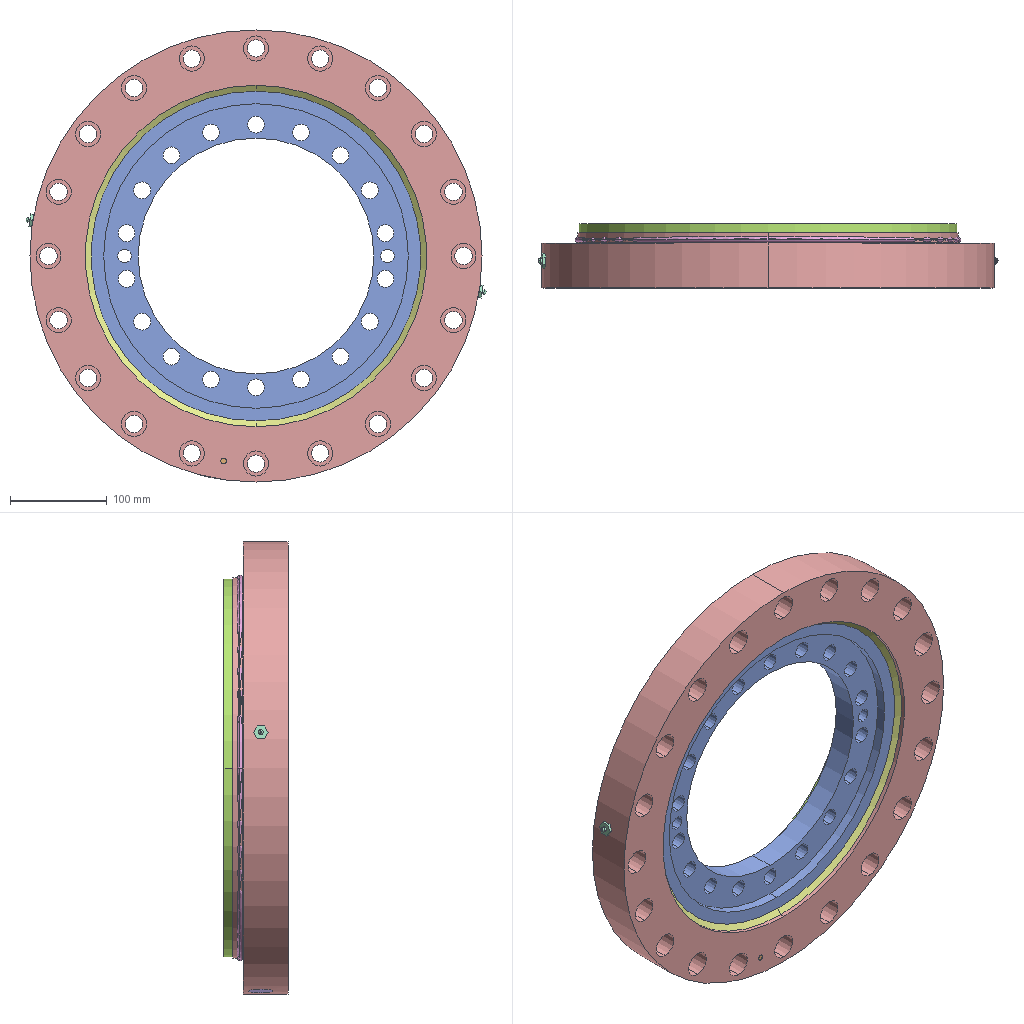Assembly | SolidWorks | 12 different items | 36 placed | box 474 x 66 x 466 mm
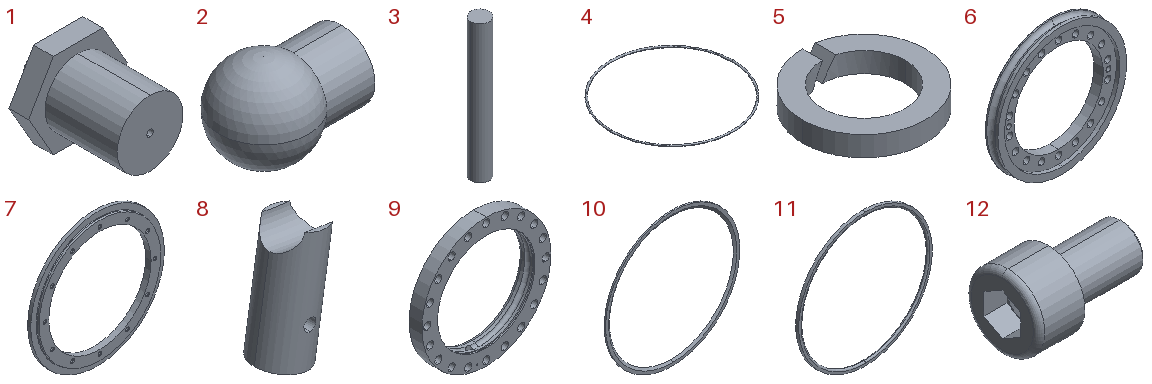Parts list (item | quantity | size | volume | features):
1 | x2 | 15 x 18 x 12.99 mm | 1356 mm3 | features Fillet 1, ICE 1, Revolution 1
2 | x1 | 27.386 x 20 x 20 mm | 5453 mm3 | features Revolution 2
3 | x1 | 6 x 6 x 45 mm | 1272 mm3 | features Extrusion 1
4 | x2 | 375.6 x 375.6 x 5.3 mm | 25665 mm3 | features RefAxis 1, Sweep 1
5 | x12 | 22.1 x 22.1 x 3.6 mm | 726.172 mm3 | features Cut 1, Extrusion 1
6 | x1 | 354.4 x 40 x 354.4 mm | 1222864 mm3 | features HoleWzd 3, CirPattern 2, RefAxis 1, Revolution 1
7 | x1 | 389 x 16 x 389 mm | 600136 mm3 | features CirPattern 1, Fillet 1, HoleWzd 1, RefAxis 1, Revolution 1
8 | x1 | 31.917 x 25 x 59.146 mm | 23195 mm3 | features HoleWzd 2, RefAxis 2, 3DProfileFeature 1, CirPattern 1, ICE 1, Revolution 1
9 | x1 | 466 x 57 x 466 mm | 2930059 mm3 | features ICE 2, CirPattern 1, HoleWzd 1, RefAxis 1, Revolution 1
10 | x1 | 368 x 4 x 368 mm | 49310 mm3 | features Revolution 1
11 | x1 | 354.4 x 8 x 354.4 mm | 80993 mm3 | features Revolution 1
12 | x12 | 26 x 16 x 16 mm | 2933 mm3 | features Fillet 2, RevCut 2, Boss 1, Chamfer 1, Cut 1, Extrusion 1, LPattern 1
Mates (type | each side: item.copy, entity, surface, feature):
Concentric | 9.1 face cylinder Revolve1 | 6.1 face cylinder Revolve1
DistanceDim | 6.1 face plane Revolve1 | 9.1 face plane Revolve1
Coincident | 9.1 plane | 6.1 plane
Concentric | 9.1 face cylinder Revolve1 | 7.1 face cylinder Revolve1
Concentric | 6.1 face cylinder CirPattern1 | 7.1 face cylinder CirPattern1
Coincident | 9.1 face plane Revolve1 | 7.1 face plane Revolve1
Tangent | 9.1 face plane Revolve1 | 4.1 face torus Sweep1
Coincident | 9.1 plane | 4.1 plane | 2 times
Tangent | 9.1 face plane Revolve1 | 4.2 face torus Sweep1
Coincident | 9.1 plane | 4.2 plane | 2 times
Concentric | 9.1 face cylinder Cut-Extrude3 | 3.1 face cylinder Boss-Extrude1
Coincident | 9.1 face plane Revolve1 | 3.1 face plane Boss-Extrude1
Parallel | 9.1 plane | 3.1 plane
Concentric | 3.1 face cylinder Boss-Extrude1 | 8.1 face cylinder Ø6.0 (6) Diameter Hole1
Concentric | 9.1 face cylinder Cut-Extrude2 | 8.1 face cylinder Cut-Extrude2
Parallel | 6.1 face cylinder Revolve1 | 11.1 face cylinder Revolve1
Concentric | 6.1 face cylinder Revolve1 | 11.1 face cylinder Revolve1
Coincident | 6.1 face plane Revolve1 | 11.1 face plane Revolve1
Coincident | 6.1 plane | 11.1 plane
Concentric | 7.1 face cylinder CirPattern1 | 5.1 face cylinder Base-Extrude
Coincident | 7.1 face plane CirPattern1 | 5.1 face plane Base-Extrude
Parallel | 9.1 plane | 5.1 plane
Concentric | 7.1 face cylinder CirPattern1 | 12.1 face cylinder BaseBody
Coincident | 5.1 face plane Base-Extrude | 12.1 face plane BaseHead
Parallel | 9.1 plane | 12.1 plane
Concentric | 9.1 face cylinder Revolve1 | 10.1 face cylinder Revolve1
Coincident | 9.1 face plane Revolve1 | 10.1 face plane Revolve1
Coincident | 9.1 plane | 10.1 plane
DistanceDim | 2.1 plane | 6.1 plane
Coincident | 6.1 plane | 2.1 plane
DistanceDim | 2.1 plane | 11.1 face plane Revolve1
Tangent | 9.1 face cylinder Revolve1 | 1.1 face plane Revolve1
Coincident | 9.1 plane | 1.1 plane
DistanceDim | 1.1 plane | 9.1 face plane Revolve1